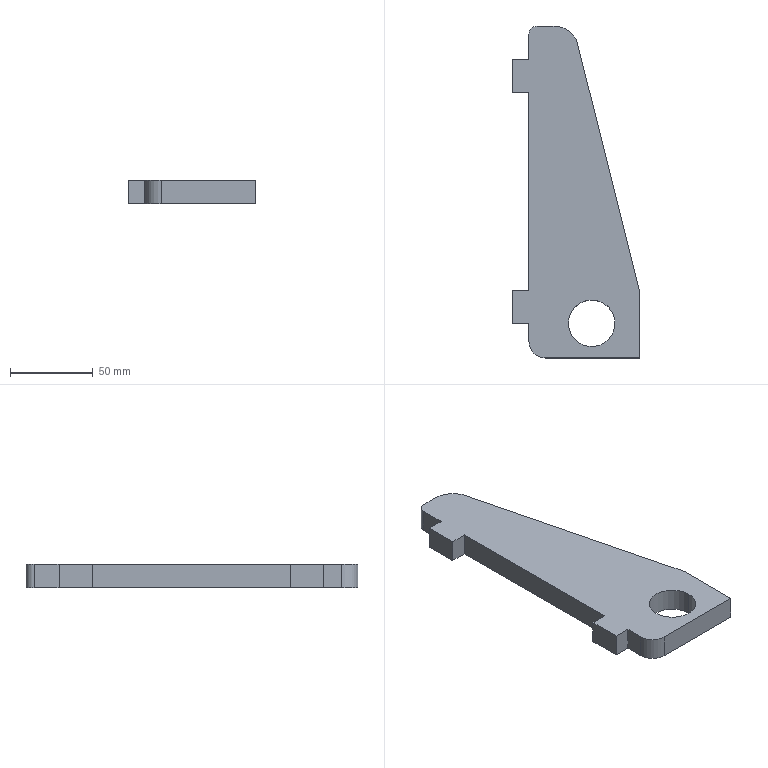Part | SolidWorks | features Extrusion 1 | 1 solid | 20 faces | box 76.998 x 201 x 14 mm | volume 139252 mm3 | plane 15 | cylinder 5 | commonest cylinder face diameters 28.2 x2 10 x1 20 x1 30 x1
STEP:
#1=CARTESIAN_POINT('',(33.9,21.,14.));
#2=VERTEX_POINT('',#1);
#3=CARTESIAN_POINT('',(62.1,21.,14.));
#4=VERTEX_POINT('',#3);
#5=CARTESIAN_POINT('',(48.,21.,14.));
#6=DIRECTION('',(0.,0.,1.));
#7=DIRECTION('',(1.,0.,0.));
#8=AXIS2_PLACEMENT_3D('',#5,#6,#7);
#9=CIRCLE('',#8,14.1);
#10=EDGE_CURVE('',#2,#4,#9,.T.);
#11=ORIENTED_EDGE('',*,*,#10,.T.);
#12=CARTESIAN_POINT('',(62.1,21.,0.));
#13=VERTEX_POINT('',#12);
#14=CARTESIAN_POINT('',(62.1,21.,14.));
#15=DIRECTION('',(0.,0.,-1.));
#16=VECTOR('',#15,1000.);
#17=LINE('',#14,#16);
#18=EDGE_CURVE('',#4,#13,#17,.T.);
#19=ORIENTED_EDGE('',*,*,#18,.T.);
#20=CARTESIAN_POINT('',(33.9,21.,0.));
#21=VERTEX_POINT('',#20);
#22=CARTESIAN_POINT('',(48.,21.,0.));
#23=DIRECTION('',(0.,0.,1.));
#24=DIRECTION('',(1.,0.,0.));
#25=AXIS2_PLACEMENT_3D('',#22,#23,#24);
#26=CIRCLE('',#25,14.1);
#27=EDGE_CURVE('',#21,#13,#26,.T.);
#28=ORIENTED_EDGE('',*,*,#27,.F.);
#29=CARTESIAN_POINT('',(33.9,21.,14.));
#30=DIRECTION('',(0.,0.,-1.));
#31=VECTOR('',#30,1000.);
#32=LINE('',#29,#31);
#33=EDGE_CURVE('',#2,#21,#32,.T.);
#34=ORIENTED_EDGE('',*,*,#33,.F.);
#35=EDGE_LOOP('',(#11,#19,#28,#34));
#36=FACE_OUTER_BOUND('',#35,.T.);
#37=CARTESIAN_POINT('',(48.,21.,14.));
#38=DIRECTION('',(0.,0.,-1.));
#39=DIRECTION('',(-1.,0.,0.));
#40=AXIS2_PLACEMENT_3D('',#37,#38,#39);
#41=CYLINDRICAL_SURFACE('',#40,14.1);
#42=ADVANCED_FACE('',(#36),#41,.F.);
#43=CARTESIAN_POINT('',(10.,10.,14.));
#44=VERTEX_POINT('',#43);
#45=CARTESIAN_POINT('',(20.,0.,14.));
#46=VERTEX_POINT('',#45);
#47=CARTESIAN_POINT('',(20.,10.,14.));
#48=DIRECTION('',(0.,0.,1.));
#49=DIRECTION('',(1.,0.,0.));
#50=AXIS2_PLACEMENT_3D('',#47,#48,#49);
#51=CIRCLE('',#50,10.);
#52=EDGE_CURVE('',#44,#46,#51,.T.);
#53=ORIENTED_EDGE('',*,*,#52,.T.);
#54=CARTESIAN_POINT('',(76.998,0.,14.));
#55=VERTEX_POINT('',#54);
#56=CARTESIAN_POINT('',(20.,0.,14.));
#57=DIRECTION('',(1.,0.,0.));
#58=VECTOR('',#57,1000.);
#59=LINE('',#56,#58);
#60=EDGE_CURVE('',#46,#55,#59,.T.);
#61=ORIENTED_EDGE('',*,*,#60,.T.);
#62=CARTESIAN_POINT('',(76.998,40.,14.));
#63=VERTEX_POINT('',#62);
#64=CARTESIAN_POINT('',(76.998,0.,14.));
#65=DIRECTION('',(0.,1.,0.));
#66=VECTOR('',#65,1000.);
#67=LINE('',#64,#66);
#68=EDGE_CURVE('',#55,#63,#67,.T.);
#69=ORIENTED_EDGE('',*,*,#68,.T.);
#70=CARTESIAN_POINT('',(38.941,192.038,14.));
#71=VERTEX_POINT('',#70);
#72=CARTESIAN_POINT('',(76.998,40.,14.));
#73=DIRECTION('',(-0.2428,0.9701,0.));
#74=VECTOR('',#73,1000.);
#75=LINE('',#72,#74);
#76=EDGE_CURVE('',#63,#71,#75,.T.);
#77=ORIENTED_EDGE('',*,*,#76,.T.);
#78=CARTESIAN_POINT('',(25.21,201.,14.));
#79=VERTEX_POINT('',#78);
#80=CARTESIAN_POINT('',(25.21,186.,14.));
#81=DIRECTION('',(0.,0.,1.));
#82=DIRECTION('',(1.,0.,0.));
#83=AXIS2_PLACEMENT_3D('',#80,#81,#82);
#84=CIRCLE('',#83,15.);
#85=EDGE_CURVE('',#71,#79,#84,.T.);
#86=ORIENTED_EDGE('',*,*,#85,.T.);
#87=CARTESIAN_POINT('',(15.,201.,14.));
#88=VERTEX_POINT('',#87);
#89=CARTESIAN_POINT('',(15.,201.,14.));
#90=DIRECTION('',(-1.,0.,0.));
#91=VECTOR('',#90,1000.);
#92=LINE('',#89,#91);
#93=EDGE_CURVE('',#79,#88,#92,.T.);
#94=ORIENTED_EDGE('',*,*,#93,.T.);
#95=CARTESIAN_POINT('',(10.,196.,14.));
#96=VERTEX_POINT('',#95);
#97=CARTESIAN_POINT('',(15.,196.,14.));
#98=DIRECTION('',(0.,0.,1.));
#99=DIRECTION('',(1.,0.,0.));
#100=AXIS2_PLACEMENT_3D('',#97,#98,#99);
#101=CIRCLE('',#100,5.);
#102=EDGE_CURVE('',#88,#96,#101,.T.);
#103=ORIENTED_EDGE('',*,*,#102,.T.);
#104=CARTESIAN_POINT('',(10.,181.,14.));
#105=VERTEX_POINT('',#104);
#106=CARTESIAN_POINT('',(10.,181.,14.));
#107=DIRECTION('',(0.,-1.,0.));
#108=VECTOR('',#107,1000.);
#109=LINE('',#106,#108);
#110=EDGE_CURVE('',#96,#105,#109,.T.);
#111=ORIENTED_EDGE('',*,*,#110,.T.);
#112=CARTESIAN_POINT('',(0.,181.,14.));
#113=VERTEX_POINT('',#112);
#114=CARTESIAN_POINT('',(10.,181.,14.));
#115=DIRECTION('',(-1.,0.,0.));
#116=VECTOR('',#115,1000.);
#117=LINE('',#114,#116);
#118=EDGE_CURVE('',#105,#113,#117,.T.);
#119=ORIENTED_EDGE('',*,*,#118,.T.);
#120=CARTESIAN_POINT('',(0.,161.,14.));
#121=VERTEX_POINT('',#120);
#122=CARTESIAN_POINT('',(0.,181.,14.));
#123=DIRECTION('',(0.,-1.,0.));
#124=VECTOR('',#123,1000.);
#125=LINE('',#122,#124);
#126=EDGE_CURVE('',#113,#121,#125,.T.);
#127=ORIENTED_EDGE('',*,*,#126,.T.);
#128=CARTESIAN_POINT('',(10.,161.,14.));
#129=VERTEX_POINT('',#128);
#130=CARTESIAN_POINT('',(0.,161.,14.));
#131=DIRECTION('',(1.,0.,0.));
#132=VECTOR('',#131,1000.);
#133=LINE('',#130,#132);
#134=EDGE_CURVE('',#121,#129,#133,.T.);
#135=ORIENTED_EDGE('',*,*,#134,.T.);
#136=CARTESIAN_POINT('',(10.,41.,14.));
#137=VERTEX_POINT('',#136);
#138=CARTESIAN_POINT('',(10.,161.,14.));
#139=DIRECTION('',(0.,-1.,0.));
#140=VECTOR('',#139,1000.);
#141=LINE('',#138,#140);
#142=EDGE_CURVE('',#129,#137,#141,.T.);
#143=ORIENTED_EDGE('',*,*,#142,.T.);
#144=CARTESIAN_POINT('',(0.,41.,14.));
#145=VERTEX_POINT('',#144);
#146=CARTESIAN_POINT('',(0.,41.,14.));
#147=DIRECTION('',(-1.,0.,0.));
#148=VECTOR('',#147,1000.);
#149=LINE('',#146,#148);
#150=EDGE_CURVE('',#137,#145,#149,.T.);
#151=ORIENTED_EDGE('',*,*,#150,.T.);
#152=CARTESIAN_POINT('',(0.,21.,14.));
#153=VERTEX_POINT('',#152);
#154=CARTESIAN_POINT('',(0.,21.,14.));
#155=DIRECTION('',(0.,-1.,0.));
#156=VECTOR('',#155,1000.);
#157=LINE('',#154,#156);
#158=EDGE_CURVE('',#145,#153,#157,.T.);
#159=ORIENTED_EDGE('',*,*,#158,.T.);
#160=CARTESIAN_POINT('',(10.,21.,14.));
#161=VERTEX_POINT('',#160);
#162=CARTESIAN_POINT('',(10.,21.,14.));
#163=DIRECTION('',(1.,0.,0.));
#164=VECTOR('',#163,1000.);
#165=LINE('',#162,#164);
#166=EDGE_CURVE('',#153,#161,#165,.T.);
#167=ORIENTED_EDGE('',*,*,#166,.T.);
#168=CARTESIAN_POINT('',(10.,10.,14.));
#169=DIRECTION('',(0.,-1.,0.));
#170=VECTOR('',#169,1000.);
#171=LINE('',#168,#170);
#172=EDGE_CURVE('',#161,#44,#171,.T.);
#173=ORIENTED_EDGE('',*,*,#172,.T.);
#174=EDGE_LOOP('',(#53,#61,#69,#77,#86,#94,#103,#111,#119,#127,#135,#143,#151,#159,#167,#173));
#175=FACE_OUTER_BOUND('',#174,.T.);
#176=ORIENTED_EDGE('',*,*,#10,.F.);
#177=CARTESIAN_POINT('',(48.,21.,14.));
#178=DIRECTION('',(0.,0.,1.));
#179=DIRECTION('',(1.,0.,0.));
#180=AXIS2_PLACEMENT_3D('',#177,#178,#179);
#181=CIRCLE('',#180,14.1);
#182=EDGE_CURVE('',#4,#2,#181,.T.);
#183=ORIENTED_EDGE('',*,*,#182,.F.);
#184=EDGE_LOOP('',(#176,#183));
#185=FACE_BOUND('',#184,.T.);
#186=CARTESIAN_POINT('',(20.,10.,14.));
#187=DIRECTION('',(0.,0.,1.));
#188=DIRECTION('',(1.,0.,0.));
#189=AXIS2_PLACEMENT_3D('',#186,#187,#188);
#190=PLANE('',#189);
#191=ADVANCED_FACE('',(#175,#185),#190,.T.);
#192=CARTESIAN_POINT('',(10.,10.,0.));
#193=VERTEX_POINT('',#192);
#194=CARTESIAN_POINT('',(20.,0.,0.));
#195=VERTEX_POINT('',#194);
#196=CARTESIAN_POINT('',(20.,10.,0.));
#197=DIRECTION('',(0.,0.,1.));
#198=DIRECTION('',(1.,0.,0.));
#199=AXIS2_PLACEMENT_3D('',#196,#197,#198);
#200=CIRCLE('',#199,10.);
#201=EDGE_CURVE('',#193,#195,#200,.T.);
#202=ORIENTED_EDGE('',*,*,#201,.F.);
#203=CARTESIAN_POINT('',(10.,21.,0.));
#204=VERTEX_POINT('',#203);
#205=CARTESIAN_POINT('',(10.,10.,0.));
#206=DIRECTION('',(0.,-1.,0.));
#207=VECTOR('',#206,1000.);
#208=LINE('',#205,#207);
#209=EDGE_CURVE('',#204,#193,#208,.T.);
#210=ORIENTED_EDGE('',*,*,#209,.F.);
#211=CARTESIAN_POINT('',(0.,21.,0.));
#212=VERTEX_POINT('',#211);
#213=CARTESIAN_POINT('',(10.,21.,0.));
#214=DIRECTION('',(1.,0.,0.));
#215=VECTOR('',#214,1000.);
#216=LINE('',#213,#215);
#217=EDGE_CURVE('',#212,#204,#216,.T.);
#218=ORIENTED_EDGE('',*,*,#217,.F.);
#219=CARTESIAN_POINT('',(0.,41.,0.));
#220=VERTEX_POINT('',#219);
#221=CARTESIAN_POINT('',(0.,21.,0.));
#222=DIRECTION('',(0.,-1.,0.));
#223=VECTOR('',#222,1000.);
#224=LINE('',#221,#223);
#225=EDGE_CURVE('',#220,#212,#224,.T.);
#226=ORIENTED_EDGE('',*,*,#225,.F.);
#227=CARTESIAN_POINT('',(10.,41.,0.));
#228=VERTEX_POINT('',#227);
#229=CARTESIAN_POINT('',(0.,41.,0.));
#230=DIRECTION('',(-1.,0.,0.));
#231=VECTOR('',#230,1000.);
#232=LINE('',#229,#231);
#233=EDGE_CURVE('',#228,#220,#232,.T.);
#234=ORIENTED_EDGE('',*,*,#233,.F.);
#235=CARTESIAN_POINT('',(10.,161.,0.));
#236=VERTEX_POINT('',#235);
#237=CARTESIAN_POINT('',(10.,101.,0.));
#238=DIRECTION('',(0.,-1.,0.));
#239=VECTOR('',#238,1000.);
#240=LINE('',#237,#239);
#241=EDGE_CURVE('',#236,#228,#240,.T.);
#242=ORIENTED_EDGE('',*,*,#241,.F.);
#243=CARTESIAN_POINT('',(0.,161.,0.));
#244=VERTEX_POINT('',#243);
#245=CARTESIAN_POINT('',(0.,161.,0.));
#246=DIRECTION('',(1.,0.,0.));
#247=VECTOR('',#246,1000.);
#248=LINE('',#245,#247);
#249=EDGE_CURVE('',#244,#236,#248,.T.);
#250=ORIENTED_EDGE('',*,*,#249,.F.);
#251=CARTESIAN_POINT('',(0.,181.,0.));
#252=VERTEX_POINT('',#251);
#253=CARTESIAN_POINT('',(0.,181.,0.));
#254=DIRECTION('',(0.,-1.,0.));
#255=VECTOR('',#254,1000.);
#256=LINE('',#253,#255);
#257=EDGE_CURVE('',#252,#244,#256,.T.);
#258=ORIENTED_EDGE('',*,*,#257,.F.);
#259=CARTESIAN_POINT('',(10.,181.,0.));
#260=VERTEX_POINT('',#259);
#261=CARTESIAN_POINT('',(10.,181.,0.));
#262=DIRECTION('',(-1.,0.,0.));
#263=VECTOR('',#262,1000.);
#264=LINE('',#261,#263);
#265=EDGE_CURVE('',#260,#252,#264,.T.);
#266=ORIENTED_EDGE('',*,*,#265,.F.);
#267=CARTESIAN_POINT('',(10.,196.,0.));
#268=VERTEX_POINT('',#267);
#269=CARTESIAN_POINT('',(10.,181.,0.));
#270=DIRECTION('',(0.,-1.,0.));
#271=VECTOR('',#270,1000.);
#272=LINE('',#269,#271);
#273=EDGE_CURVE('',#268,#260,#272,.T.);
#274=ORIENTED_EDGE('',*,*,#273,.F.);
#275=CARTESIAN_POINT('',(15.,201.,0.));
#276=VERTEX_POINT('',#275);
#277=CARTESIAN_POINT('',(15.,196.,0.));
#278=DIRECTION('',(0.,0.,1.));
#279=DIRECTION('',(1.,0.,0.));
#280=AXIS2_PLACEMENT_3D('',#277,#278,#279);
#281=CIRCLE('',#280,5.);
#282=EDGE_CURVE('',#276,#268,#281,.T.);
#283=ORIENTED_EDGE('',*,*,#282,.F.);
#284=CARTESIAN_POINT('',(25.21,201.,0.));
#285=VERTEX_POINT('',#284);
#286=CARTESIAN_POINT('',(15.,201.,0.));
#287=DIRECTION('',(-1.,0.,0.));
#288=VECTOR('',#287,1000.);
#289=LINE('',#286,#288);
#290=EDGE_CURVE('',#285,#276,#289,.T.);
#291=ORIENTED_EDGE('',*,*,#290,.F.);
#292=CARTESIAN_POINT('',(38.941,192.038,0.));
#293=VERTEX_POINT('',#292);
#294=CARTESIAN_POINT('',(25.21,186.,0.));
#295=DIRECTION('',(0.,0.,1.));
#296=DIRECTION('',(1.,0.,0.));
#297=AXIS2_PLACEMENT_3D('',#294,#295,#296);
#298=CIRCLE('',#297,15.);
#299=EDGE_CURVE('',#293,#285,#298,.T.);
#300=ORIENTED_EDGE('',*,*,#299,.F.);
#301=CARTESIAN_POINT('',(76.998,40.,0.));
#302=VERTEX_POINT('',#301);
#303=CARTESIAN_POINT('',(76.998,40.,0.));
#304=DIRECTION('',(-0.2428,0.9701,0.));
#305=VECTOR('',#304,1000.);
#306=LINE('',#303,#305);
#307=EDGE_CURVE('',#302,#293,#306,.T.);
#308=ORIENTED_EDGE('',*,*,#307,.F.);
#309=CARTESIAN_POINT('',(76.998,0.,0.));
#310=VERTEX_POINT('',#309);
#311=CARTESIAN_POINT('',(76.998,30.,0.));
#312=DIRECTION('',(0.,1.,0.));
#313=VECTOR('',#312,1000.);
#314=LINE('',#311,#313);
#315=EDGE_CURVE('',#310,#302,#314,.T.);
#316=ORIENTED_EDGE('',*,*,#315,.F.);
#317=CARTESIAN_POINT('',(20.,0.,0.));
#318=DIRECTION('',(1.,0.,0.));
#319=VECTOR('',#318,1000.);
#320=LINE('',#317,#319);
#321=EDGE_CURVE('',#195,#310,#320,.T.);
#322=ORIENTED_EDGE('',*,*,#321,.F.);
#323=EDGE_LOOP('',(#202,#210,#218,#226,#234,#242,#250,#258,#266,#274,#283,#291,#300,#308,#316,#322));
#324=FACE_OUTER_BOUND('',#323,.T.);
#325=ORIENTED_EDGE('',*,*,#27,.T.);
#326=CARTESIAN_POINT('',(48.,21.,0.));
#327=DIRECTION('',(0.,0.,1.));
#328=DIRECTION('',(1.,0.,0.));
#329=AXIS2_PLACEMENT_3D('',#326,#327,#328);
#330=CIRCLE('',#329,14.1);
#331=EDGE_CURVE('',#13,#21,#330,.T.);
#332=ORIENTED_EDGE('',*,*,#331,.T.);
#333=EDGE_LOOP('',(#325,#332));
#334=FACE_BOUND('',#333,.T.);
#335=CARTESIAN_POINT('',(20.,10.,0.));
#336=DIRECTION('',(0.,0.,1.));
#337=DIRECTION('',(1.,0.,0.));
#338=AXIS2_PLACEMENT_3D('',#335,#336,#337);
#339=PLANE('',#338);
#340=ADVANCED_FACE('',(#324,#334),#339,.F.);
#341=ORIENTED_EDGE('',*,*,#201,.T.);
#342=CARTESIAN_POINT('',(20.,0.,14.));
#343=DIRECTION('',(0.,0.,-1.));
#344=VECTOR('',#343,1000.);
#345=LINE('',#342,#344);
#346=EDGE_CURVE('',#46,#195,#345,.T.);
#347=ORIENTED_EDGE('',*,*,#346,.F.);
#348=ORIENTED_EDGE('',*,*,#52,.F.);
#349=CARTESIAN_POINT('',(10.,10.,14.));
#350=DIRECTION('',(0.,0.,-1.));
#351=VECTOR('',#350,1000.);
#352=LINE('',#349,#351);
#353=EDGE_CURVE('',#44,#193,#352,.T.);
#354=ORIENTED_EDGE('',*,*,#353,.T.);
#355=EDGE_LOOP('',(#341,#347,#348,#354));
#356=FACE_OUTER_BOUND('',#355,.T.);
#357=CARTESIAN_POINT('',(20.,10.,14.));
#358=DIRECTION('',(0.,0.,-1.));
#359=DIRECTION('',(-1.,0.,0.));
#360=AXIS2_PLACEMENT_3D('',#357,#358,#359);
#361=CYLINDRICAL_SURFACE('',#360,10.);
#362=ADVANCED_FACE('',(#356),#361,.T.);
#363=ORIENTED_EDGE('',*,*,#321,.T.);
#364=CARTESIAN_POINT('',(76.998,0.,14.));
#365=DIRECTION('',(0.,0.,-1.));
#366=VECTOR('',#365,1000.);
#367=LINE('',#364,#366);
#368=EDGE_CURVE('',#55,#310,#367,.T.);
#369=ORIENTED_EDGE('',*,*,#368,.F.);
#370=ORIENTED_EDGE('',*,*,#60,.F.);
#371=ORIENTED_EDGE('',*,*,#346,.T.);
#372=EDGE_LOOP('',(#363,#369,#370,#371));
#373=FACE_OUTER_BOUND('',#372,.T.);
#374=CARTESIAN_POINT('',(20.,0.,14.));
#375=DIRECTION('',(0.,1.,0.));
#376=DIRECTION('',(0.,0.,1.));
#377=AXIS2_PLACEMENT_3D('',#374,#375,#376);
#378=PLANE('',#377);
#379=ADVANCED_FACE('',(#373),#378,.F.);
#380=ORIENTED_EDGE('',*,*,#315,.T.);
#381=CARTESIAN_POINT('',(76.998,40.,14.));
#382=DIRECTION('',(0.,0.,-1.));
#383=VECTOR('',#382,1000.);
#384=LINE('',#381,#383);
#385=EDGE_CURVE('',#63,#302,#384,.T.);
#386=ORIENTED_EDGE('',*,*,#385,.F.);
#387=ORIENTED_EDGE('',*,*,#68,.F.);
#388=ORIENTED_EDGE('',*,*,#368,.T.);
#389=EDGE_LOOP('',(#380,#386,#387,#388));
#390=FACE_OUTER_BOUND('',#389,.T.);
#391=CARTESIAN_POINT('',(76.998,30.,14.));
#392=DIRECTION('',(-1.,0.,0.));
#393=DIRECTION('',(0.,0.,1.));
#394=AXIS2_PLACEMENT_3D('',#391,#392,#393);
#395=PLANE('',#394);
#396=ADVANCED_FACE('',(#390),#395,.F.);
#397=ORIENTED_EDGE('',*,*,#307,.T.);
#398=CARTESIAN_POINT('',(38.941,192.038,14.));
#399=DIRECTION('',(0.,0.,-1.));
#400=VECTOR('',#399,1000.);
#401=LINE('',#398,#400);
#402=EDGE_CURVE('',#71,#293,#401,.T.);
#403=ORIENTED_EDGE('',*,*,#402,.F.);
#404=ORIENTED_EDGE('',*,*,#76,.F.);
#405=ORIENTED_EDGE('',*,*,#385,.T.);
#406=EDGE_LOOP('',(#397,#403,#404,#405));
#407=FACE_OUTER_BOUND('',#406,.T.);
#408=CARTESIAN_POINT('',(76.998,40.,14.));
#409=DIRECTION('',(-0.9701,-0.2428,0.));
#410=DIRECTION('',(0.2428,-0.9701,0.));
#411=AXIS2_PLACEMENT_3D('',#408,#409,#410);
#412=PLANE('',#411);
#413=ADVANCED_FACE('',(#407),#412,.F.);
#414=ORIENTED_EDGE('',*,*,#299,.T.);
#415=CARTESIAN_POINT('',(25.21,201.,14.));
#416=DIRECTION('',(0.,0.,-1.));
#417=VECTOR('',#416,1000.);
#418=LINE('',#415,#417);
#419=EDGE_CURVE('',#79,#285,#418,.T.);
#420=ORIENTED_EDGE('',*,*,#419,.F.);
#421=ORIENTED_EDGE('',*,*,#85,.F.);
#422=ORIENTED_EDGE('',*,*,#402,.T.);
#423=EDGE_LOOP('',(#414,#420,#421,#422));
#424=FACE_OUTER_BOUND('',#423,.T.);
#425=CARTESIAN_POINT('',(25.21,186.,14.));
#426=DIRECTION('',(0.,0.,-1.));
#427=DIRECTION('',(-1.,0.,0.));
#428=AXIS2_PLACEMENT_3D('',#425,#426,#427);
#429=CYLINDRICAL_SURFACE('',#428,15.);
#430=ADVANCED_FACE('',(#424),#429,.T.);
#431=ORIENTED_EDGE('',*,*,#290,.T.);
#432=CARTESIAN_POINT('',(15.,201.,14.));
#433=DIRECTION('',(0.,0.,-1.));
#434=VECTOR('',#433,1000.);
#435=LINE('',#432,#434);
#436=EDGE_CURVE('',#88,#276,#435,.T.);
#437=ORIENTED_EDGE('',*,*,#436,.F.);
#438=ORIENTED_EDGE('',*,*,#93,.F.);
#439=ORIENTED_EDGE('',*,*,#419,.T.);
#440=EDGE_LOOP('',(#431,#437,#438,#439));
#441=FACE_OUTER_BOUND('',#440,.T.);
#442=CARTESIAN_POINT('',(15.,201.,14.));
#443=DIRECTION('',(0.,-1.,0.));
#444=DIRECTION('',(1.,0.,0.));
#445=AXIS2_PLACEMENT_3D('',#442,#443,#444);
#446=PLANE('',#445);
#447=ADVANCED_FACE('',(#441),#446,.F.);
#448=ORIENTED_EDGE('',*,*,#282,.T.);
#449=CARTESIAN_POINT('',(10.,196.,14.));
#450=DIRECTION('',(0.,0.,-1.));
#451=VECTOR('',#450,1000.);
#452=LINE('',#449,#451);
#453=EDGE_CURVE('',#96,#268,#452,.T.);
#454=ORIENTED_EDGE('',*,*,#453,.F.);
#455=ORIENTED_EDGE('',*,*,#102,.F.);
#456=ORIENTED_EDGE('',*,*,#436,.T.);
#457=EDGE_LOOP('',(#448,#454,#455,#456));
#458=FACE_OUTER_BOUND('',#457,.T.);
#459=CARTESIAN_POINT('',(15.,196.,14.));
#460=DIRECTION('',(0.,0.,-1.));
#461=DIRECTION('',(-1.,0.,0.));
#462=AXIS2_PLACEMENT_3D('',#459,#460,#461);
#463=CYLINDRICAL_SURFACE('',#462,5.);
#464=ADVANCED_FACE('',(#458),#463,.T.);
#465=ORIENTED_EDGE('',*,*,#273,.T.);
#466=CARTESIAN_POINT('',(10.,181.,14.));
#467=DIRECTION('',(0.,0.,-1.));
#468=VECTOR('',#467,1000.);
#469=LINE('',#466,#468);
#470=EDGE_CURVE('',#105,#260,#469,.T.);
#471=ORIENTED_EDGE('',*,*,#470,.F.);
#472=ORIENTED_EDGE('',*,*,#110,.F.);
#473=ORIENTED_EDGE('',*,*,#453,.T.);
#474=EDGE_LOOP('',(#465,#471,#472,#473));
#475=FACE_OUTER_BOUND('',#474,.T.);
#476=CARTESIAN_POINT('',(10.,181.,14.));
#477=DIRECTION('',(1.,0.,0.));
#478=DIRECTION('',(0.,0.,-1.));
#479=AXIS2_PLACEMENT_3D('',#476,#477,#478);
#480=PLANE('',#479);
#481=ADVANCED_FACE('',(#475),#480,.F.);
#482=ORIENTED_EDGE('',*,*,#265,.T.);
#483=CARTESIAN_POINT('',(0.,181.,14.));
#484=DIRECTION('',(0.,0.,-1.));
#485=VECTOR('',#484,1000.);
#486=LINE('',#483,#485);
#487=EDGE_CURVE('',#113,#252,#486,.T.);
#488=ORIENTED_EDGE('',*,*,#487,.F.);
#489=ORIENTED_EDGE('',*,*,#118,.F.);
#490=ORIENTED_EDGE('',*,*,#470,.T.);
#491=EDGE_LOOP('',(#482,#488,#489,#490));
#492=FACE_OUTER_BOUND('',#491,.T.);
#493=CARTESIAN_POINT('',(10.,181.,14.));
#494=DIRECTION('',(0.,-1.,0.));
#495=DIRECTION('',(0.,0.,-1.));
#496=AXIS2_PLACEMENT_3D('',#493,#494,#495);
#497=PLANE('',#496);
#498=ADVANCED_FACE('',(#492),#497,.F.);
#499=ORIENTED_EDGE('',*,*,#257,.T.);
#500=CARTESIAN_POINT('',(0.,161.,14.));
#501=DIRECTION('',(0.,0.,-1.));
#502=VECTOR('',#501,1000.);
#503=LINE('',#500,#502);
#504=EDGE_CURVE('',#121,#244,#503,.T.);
#505=ORIENTED_EDGE('',*,*,#504,.F.);
#506=ORIENTED_EDGE('',*,*,#126,.F.);
#507=ORIENTED_EDGE('',*,*,#487,.T.);
#508=EDGE_LOOP('',(#499,#505,#506,#507));
#509=FACE_OUTER_BOUND('',#508,.T.);
#510=CARTESIAN_POINT('',(0.,181.,14.));
#511=DIRECTION('',(1.,0.,0.));
#512=DIRECTION('',(0.,0.,-1.));
#513=AXIS2_PLACEMENT_3D('',#510,#511,#512);
#514=PLANE('',#513);
#515=ADVANCED_FACE('',(#509),#514,.F.);
#516=ORIENTED_EDGE('',*,*,#249,.T.);
#517=CARTESIAN_POINT('',(10.,161.,14.));
#518=DIRECTION('',(0.,0.,-1.));
#519=VECTOR('',#518,1000.);
#520=LINE('',#517,#519);
#521=EDGE_CURVE('',#129,#236,#520,.T.);
#522=ORIENTED_EDGE('',*,*,#521,.F.);
#523=ORIENTED_EDGE('',*,*,#134,.F.);
#524=ORIENTED_EDGE('',*,*,#504,.T.);
#525=EDGE_LOOP('',(#516,#522,#523,#524));
#526=FACE_OUTER_BOUND('',#525,.T.);
#527=CARTESIAN_POINT('',(0.,161.,14.));
#528=DIRECTION('',(0.,1.,0.));
#529=DIRECTION('',(0.,0.,1.));
#530=AXIS2_PLACEMENT_3D('',#527,#528,#529);
#531=PLANE('',#530);
#532=ADVANCED_FACE('',(#526),#531,.F.);
#533=ORIENTED_EDGE('',*,*,#241,.T.);
#534=CARTESIAN_POINT('',(10.,41.,14.));
#535=DIRECTION('',(0.,0.,-1.));
#536=VECTOR('',#535,1000.);
#537=LINE('',#534,#536);
#538=EDGE_CURVE('',#137,#228,#537,.T.);
#539=ORIENTED_EDGE('',*,*,#538,.F.);
#540=ORIENTED_EDGE('',*,*,#142,.F.);
#541=ORIENTED_EDGE('',*,*,#521,.T.);
#542=EDGE_LOOP('',(#533,#539,#540,#541));
#543=FACE_OUTER_BOUND('',#542,.T.);
#544=CARTESIAN_POINT('',(10.,101.,14.));
#545=DIRECTION('',(1.,0.,0.));
#546=DIRECTION('',(0.,0.,-1.));
#547=AXIS2_PLACEMENT_3D('',#544,#545,#546);
#548=PLANE('',#547);
#549=ADVANCED_FACE('',(#543),#548,.F.);
#550=ORIENTED_EDGE('',*,*,#233,.T.);
#551=CARTESIAN_POINT('',(0.,41.,14.));
#552=DIRECTION('',(0.,0.,-1.));
#553=VECTOR('',#552,1000.);
#554=LINE('',#551,#553);
#555=EDGE_CURVE('',#145,#220,#554,.T.);
#556=ORIENTED_EDGE('',*,*,#555,.F.);
#557=ORIENTED_EDGE('',*,*,#150,.F.);
#558=ORIENTED_EDGE('',*,*,#538,.T.);
#559=EDGE_LOOP('',(#550,#556,#557,#558));
#560=FACE_OUTER_BOUND('',#559,.T.);
#561=CARTESIAN_POINT('',(0.,41.,14.));
#562=DIRECTION('',(0.,-1.,0.));
#563=DIRECTION('',(0.,0.,-1.));
#564=AXIS2_PLACEMENT_3D('',#561,#562,#563);
#565=PLANE('',#564);
#566=ADVANCED_FACE('',(#560),#565,.F.);
#567=ORIENTED_EDGE('',*,*,#225,.T.);
#568=CARTESIAN_POINT('',(0.,21.,14.));
#569=DIRECTION('',(0.,0.,-1.));
#570=VECTOR('',#569,1000.);
#571=LINE('',#568,#570);
#572=EDGE_CURVE('',#153,#212,#571,.T.);
#573=ORIENTED_EDGE('',*,*,#572,.F.);
#574=ORIENTED_EDGE('',*,*,#158,.F.);
#575=ORIENTED_EDGE('',*,*,#555,.T.);
#576=EDGE_LOOP('',(#567,#573,#574,#575));
#577=FACE_OUTER_BOUND('',#576,.T.);
#578=CARTESIAN_POINT('',(0.,21.,14.));
#579=DIRECTION('',(1.,0.,0.));
#580=DIRECTION('',(0.,0.,-1.));
#581=AXIS2_PLACEMENT_3D('',#578,#579,#580);
#582=PLANE('',#581);
#583=ADVANCED_FACE('',(#577),#582,.F.);
#584=ORIENTED_EDGE('',*,*,#217,.T.);
#585=CARTESIAN_POINT('',(10.,21.,14.));
#586=DIRECTION('',(0.,0.,-1.));
#587=VECTOR('',#586,1000.);
#588=LINE('',#585,#587);
#589=EDGE_CURVE('',#161,#204,#588,.T.);
#590=ORIENTED_EDGE('',*,*,#589,.F.);
#591=ORIENTED_EDGE('',*,*,#166,.F.);
#592=ORIENTED_EDGE('',*,*,#572,.T.);
#593=EDGE_LOOP('',(#584,#590,#591,#592));
#594=FACE_OUTER_BOUND('',#593,.T.);
#595=CARTESIAN_POINT('',(10.,21.,14.));
#596=DIRECTION('',(0.,1.,0.));
#597=DIRECTION('',(0.,0.,1.));
#598=AXIS2_PLACEMENT_3D('',#595,#596,#597);
#599=PLANE('',#598);
#600=ADVANCED_FACE('',(#594),#599,.F.);
#601=ORIENTED_EDGE('',*,*,#209,.T.);
#602=ORIENTED_EDGE('',*,*,#353,.F.);
#603=ORIENTED_EDGE('',*,*,#172,.F.);
#604=ORIENTED_EDGE('',*,*,#589,.T.);
#605=EDGE_LOOP('',(#601,#602,#603,#604));
#606=FACE_OUTER_BOUND('',#605,.T.);
#607=CARTESIAN_POINT('',(10.,10.,14.));
#608=DIRECTION('',(1.,0.,0.));
#609=DIRECTION('',(0.,0.,-1.));
#610=AXIS2_PLACEMENT_3D('',#607,#608,#609);
#611=PLANE('',#610);
#612=ADVANCED_FACE('',(#606),#611,.F.);
#613=ORIENTED_EDGE('',*,*,#18,.F.);
#614=ORIENTED_EDGE('',*,*,#182,.T.);
#615=ORIENTED_EDGE('',*,*,#33,.T.);
#616=ORIENTED_EDGE('',*,*,#331,.F.);
#617=EDGE_LOOP('',(#613,#614,#615,#616));
#618=FACE_OUTER_BOUND('',#617,.T.);
#619=CARTESIAN_POINT('',(48.,21.,14.));
#620=DIRECTION('',(0.,0.,-1.));
#621=DIRECTION('',(-1.,0.,0.));
#622=AXIS2_PLACEMENT_3D('',#619,#620,#621);
#623=CYLINDRICAL_SURFACE('',#622,14.1);
#624=ADVANCED_FACE('',(#618),#623,.F.);
#625=CLOSED_SHELL('',(#42,#191,#340,#362,#379,#396,#413,#430,#447,#464,#481,#498,#515,#532,#549,#566,#583,#600,#612,#624));
#626=MANIFOLD_SOLID_BREP('',#625);
#627=CARTESIAN_POINT('',(0.,0.,0.));
#628=DIRECTION('',(0.,0.,1.));
#629=DIRECTION('',(1.,0.,0.));
#630=AXIS2_PLACEMENT_3D('',#627,#628,#629);
#631=(LENGTH_UNIT()NAMED_UNIT(*)SI_UNIT(.MILLI.,.METRE.));
#632=UNCERTAINTY_MEASURE_WITH_UNIT(LENGTH_MEASURE(0.00001),#631,'','');
#633=(NAMED_UNIT(*)PLANE_ANGLE_UNIT()SI_UNIT($,.RADIAN.));
#634=(NAMED_UNIT(*)SI_UNIT($,.STERADIAN.)SOLID_ANGLE_UNIT());
#635=(GEOMETRIC_REPRESENTATION_CONTEXT(3)GLOBAL_UNCERTAINTY_ASSIGNED_CONTEXT((#632))GLOBAL_UNIT_ASSIGNED_CONTEXT((#631,#633,#634))REPRESENTATION_CONTEXT('',''));
#636=ADVANCED_BREP_SHAPE_REPRESENTATION('',(#626,#630),#635);